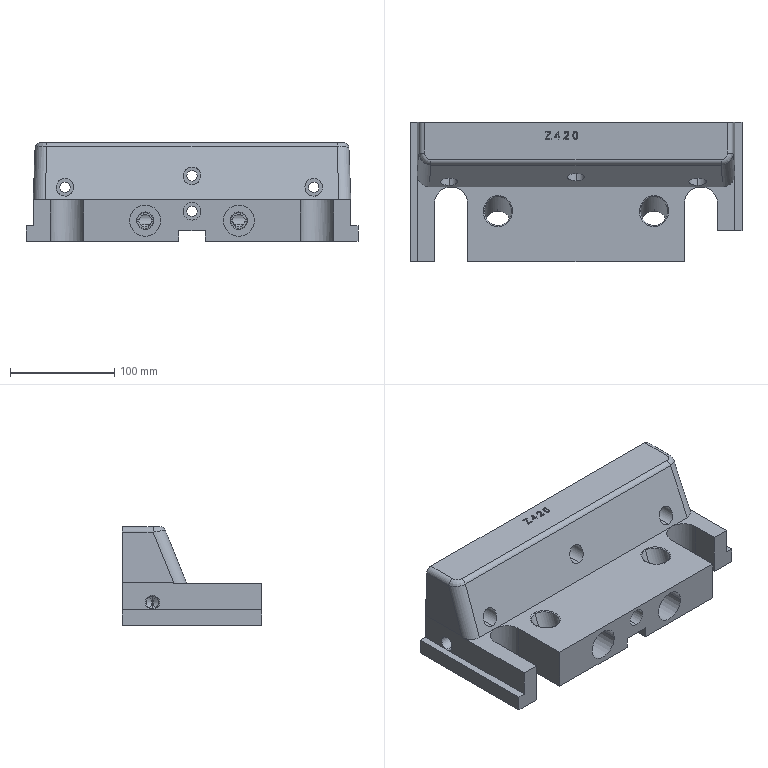Part | Creo | 1 solid | 238 faces | box 319 x 134 x 95 mm | volume 1909256 mm3 | plane 74 | cylinder 73 | other 43 | cone 30 | spline 10 | sphere 8 | commonest cylinder face diameters 12 x24 10 x8 17 x8 13 x4 14 x4 21.5 x4